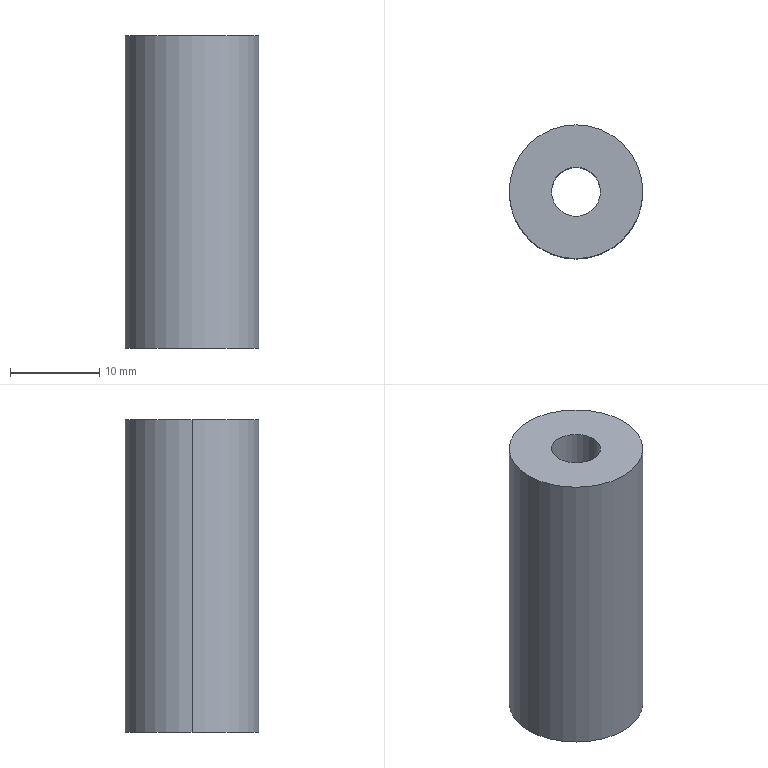Part | STEP file | track post-1 | 1 solid | 6 faces | box 15 x 15 x 35 mm | volume 5353 mm3 | cylinder 4 | plane 2 | commonest cylinder face diameters 5.5 x2 15 x2
STEP:
#1=CARTESIAN_POINT('',(0.,0.,0.));
#2=DIRECTION('',(0.,0.,1.));
#3=DIRECTION('',(1.,0.,0.));
#4=AXIS2_PLACEMENT_3D('',#1,#2,#3);
#5=CARTESIAN_POINT('',(2.75,0.,0.));
#6=VERTEX_POINT('',#5);
#7=CARTESIAN_POINT('',(2.75,0.,35.));
#8=VERTEX_POINT('',#7);
#9=CARTESIAN_POINT('',(2.75,0.,35.));
#10=DIRECTION('',(0.,0.,1.));
#11=VECTOR('',#10,1.);
#12=LINE('',#9,#11);
#13=CARTESIAN_POINT('',(0.,0.,35.));
#14=DIRECTION('',(0.,0.,1.));
#15=DIRECTION('',(1.,0.,0.));
#16=AXIS2_PLACEMENT_3D('',#13,#14,#15);
#17=CYLINDRICAL_SURFACE('',#16,2.75);
#18=CARTESIAN_POINT('',(6.283,0.));
#19=DIRECTION('',(0.,1.));
#20=VECTOR('',#19,1.);
#21=LINE('',#18,#20);
#22=(GEOMETRIC_REPRESENTATION_CONTEXT(2)PARAMETRIC_REPRESENTATION_CONTEXT()REPRESENTATION_CONTEXT('',''));
#23=DEFINITIONAL_REPRESENTATION('',(#21),#22);
#24=PCURVE('',#17,#23);
#25=CARTESIAN_POINT('',(0.,0.,35.));
#26=DIRECTION('',(0.,0.,1.));
#27=DIRECTION('',(1.,0.,0.));
#28=AXIS2_PLACEMENT_3D('',#25,#26,#27);
#29=CYLINDRICAL_SURFACE('',#28,2.75);
#30=CARTESIAN_POINT('',(0.,0.));
#31=DIRECTION('',(0.,1.));
#32=VECTOR('',#31,1.);
#33=LINE('',#30,#32);
#34=(GEOMETRIC_REPRESENTATION_CONTEXT(2)PARAMETRIC_REPRESENTATION_CONTEXT()REPRESENTATION_CONTEXT('',''));
#35=DEFINITIONAL_REPRESENTATION('',(#33),#34);
#36=PCURVE('',#29,#35);
#37=SURFACE_CURVE('',#12,(#24,#36),.PCURVE_S1.);
#38=EDGE_CURVE('',#6,#8,#37,.T.);
#39=ORIENTED_EDGE('',*,*,#38,.T.);
#40=CARTESIAN_POINT('',(-2.75,0.,35.));
#41=VERTEX_POINT('',#40);
#42=CARTESIAN_POINT('',(0.,0.,35.));
#43=DIRECTION('',(0.,0.,1.));
#44=DIRECTION('',(1.,0.,0.));
#45=AXIS2_PLACEMENT_3D('',#42,#43,#44);
#46=CIRCLE('',#45,2.75);
#47=CARTESIAN_POINT('',(0.,0.));
#48=DIRECTION('',(1.,0.));
#49=VECTOR('',#48,1.);
#50=LINE('',#47,#49);
#51=(GEOMETRIC_REPRESENTATION_CONTEXT(2)PARAMETRIC_REPRESENTATION_CONTEXT()REPRESENTATION_CONTEXT('',''));
#52=DEFINITIONAL_REPRESENTATION('',(#50),#51);
#53=PCURVE('',#17,#52);
#54=CARTESIAN_POINT('',(0.,0.,35.));
#55=DIRECTION('',(0.,0.,1.));
#56=DIRECTION('',(1.,0.,0.));
#57=AXIS2_PLACEMENT_3D('',#54,#55,#56);
#58=PLANE('',#57);
#59=CARTESIAN_POINT('',(0.,0.));
#60=DIRECTION('',(1.,0.));
#61=AXIS2_PLACEMENT_2D('',#59,#60);
#62=CIRCLE('',#61,2.75);
#63=(GEOMETRIC_REPRESENTATION_CONTEXT(2)PARAMETRIC_REPRESENTATION_CONTEXT()REPRESENTATION_CONTEXT('',''));
#64=DEFINITIONAL_REPRESENTATION('',(#62),#63);
#65=PCURVE('',#58,#64);
#66=SURFACE_CURVE('',#46,(#53,#65),.PCURVE_S1.);
#67=EDGE_CURVE('',#41,#8,#66,.T.);
#68=ORIENTED_EDGE('',*,*,#67,.F.);
#69=CARTESIAN_POINT('',(-2.75,0.,0.));
#70=VERTEX_POINT('',#69);
#71=CARTESIAN_POINT('',(-2.75,0.,35.));
#72=DIRECTION('',(0.,0.,1.));
#73=VECTOR('',#72,1.);
#74=LINE('',#71,#73);
#75=CARTESIAN_POINT('',(3.142,0.));
#76=DIRECTION('',(0.,1.));
#77=VECTOR('',#76,1.);
#78=LINE('',#75,#77);
#79=(GEOMETRIC_REPRESENTATION_CONTEXT(2)PARAMETRIC_REPRESENTATION_CONTEXT()REPRESENTATION_CONTEXT('',''));
#80=DEFINITIONAL_REPRESENTATION('',(#78),#79);
#81=PCURVE('',#17,#80);
#82=CARTESIAN_POINT('',(3.142,0.));
#83=DIRECTION('',(0.,1.));
#84=VECTOR('',#83,1.);
#85=LINE('',#82,#84);
#86=(GEOMETRIC_REPRESENTATION_CONTEXT(2)PARAMETRIC_REPRESENTATION_CONTEXT()REPRESENTATION_CONTEXT('',''));
#87=DEFINITIONAL_REPRESENTATION('',(#85),#86);
#88=PCURVE('',#29,#87);
#89=SURFACE_CURVE('',#74,(#81,#88),.PCURVE_S1.);
#90=EDGE_CURVE('',#70,#41,#89,.T.);
#91=ORIENTED_EDGE('',*,*,#90,.F.);
#92=CARTESIAN_POINT('',(0.,0.,0.));
#93=DIRECTION('',(0.,0.,1.));
#94=DIRECTION('',(1.,0.,0.));
#95=AXIS2_PLACEMENT_3D('',#92,#93,#94);
#96=CIRCLE('',#95,2.75);
#97=CARTESIAN_POINT('',(0.,-35.));
#98=DIRECTION('',(1.,0.));
#99=VECTOR('',#98,1.);
#100=LINE('',#97,#99);
#101=(GEOMETRIC_REPRESENTATION_CONTEXT(2)PARAMETRIC_REPRESENTATION_CONTEXT()REPRESENTATION_CONTEXT('',''));
#102=DEFINITIONAL_REPRESENTATION('',(#100),#101);
#103=PCURVE('',#17,#102);
#104=CARTESIAN_POINT('',(0.,0.,0.));
#105=DIRECTION('',(0.,0.,1.));
#106=DIRECTION('',(1.,0.,0.));
#107=AXIS2_PLACEMENT_3D('',#104,#105,#106);
#108=PLANE('',#107);
#109=CARTESIAN_POINT('',(0.,0.));
#110=DIRECTION('',(1.,0.));
#111=AXIS2_PLACEMENT_2D('',#109,#110);
#112=CIRCLE('',#111,2.75);
#113=(GEOMETRIC_REPRESENTATION_CONTEXT(2)PARAMETRIC_REPRESENTATION_CONTEXT()REPRESENTATION_CONTEXT('',''));
#114=DEFINITIONAL_REPRESENTATION('',(#112),#113);
#115=PCURVE('',#108,#114);
#116=SURFACE_CURVE('',#96,(#103,#115),.PCURVE_S1.);
#117=EDGE_CURVE('',#70,#6,#116,.T.);
#118=ORIENTED_EDGE('',*,*,#117,.T.);
#119=EDGE_LOOP('',(#39,#68,#91,#118));
#120=FACE_BOUND('',#119,.F.);
#121=ADVANCED_FACE('',(#120),#17,.F.);
#122=CARTESIAN_POINT('',(7.5,0.,35.));
#123=VERTEX_POINT('',#122);
#124=CARTESIAN_POINT('',(-7.5,0.,35.));
#125=VERTEX_POINT('',#124);
#126=CARTESIAN_POINT('',(0.,0.,35.));
#127=DIRECTION('',(0.,0.,1.));
#128=DIRECTION('',(1.,0.,0.));
#129=AXIS2_PLACEMENT_3D('',#126,#127,#128);
#130=CIRCLE('',#129,7.5);
#131=CARTESIAN_POINT('',(0.,0.,35.));
#132=DIRECTION('',(0.,0.,-1.));
#133=DIRECTION('',(-1.,0.,0.));
#134=AXIS2_PLACEMENT_3D('',#131,#132,#133);
#135=CYLINDRICAL_SURFACE('',#134,7.5);
#136=CARTESIAN_POINT('',(3.142,0.));
#137=DIRECTION('',(-1.,0.));
#138=VECTOR('',#137,1.);
#139=LINE('',#136,#138);
#140=(GEOMETRIC_REPRESENTATION_CONTEXT(2)PARAMETRIC_REPRESENTATION_CONTEXT()REPRESENTATION_CONTEXT('',''));
#141=DEFINITIONAL_REPRESENTATION('',(#139),#140);
#142=PCURVE('',#135,#141);
#143=CARTESIAN_POINT('',(0.,0.));
#144=DIRECTION('',(1.,0.));
#145=AXIS2_PLACEMENT_2D('',#143,#144);
#146=CIRCLE('',#145,7.5);
#147=(GEOMETRIC_REPRESENTATION_CONTEXT(2)PARAMETRIC_REPRESENTATION_CONTEXT()REPRESENTATION_CONTEXT('',''));
#148=DEFINITIONAL_REPRESENTATION('',(#146),#147);
#149=PCURVE('',#58,#148);
#150=SURFACE_CURVE('',#130,(#142,#149),.PCURVE_S1.);
#151=EDGE_CURVE('',#123,#125,#150,.T.);
#152=ORIENTED_EDGE('',*,*,#151,.F.);
#153=CARTESIAN_POINT('',(7.5,0.,0.));
#154=VERTEX_POINT('',#153);
#155=CARTESIAN_POINT('',(7.5,0.,35.));
#156=DIRECTION('',(0.,0.,-1.));
#157=VECTOR('',#156,1.);
#158=LINE('',#155,#157);
#159=CARTESIAN_POINT('',(3.142,0.));
#160=DIRECTION('',(0.,1.));
#161=VECTOR('',#160,1.);
#162=LINE('',#159,#161);
#163=(GEOMETRIC_REPRESENTATION_CONTEXT(2)PARAMETRIC_REPRESENTATION_CONTEXT()REPRESENTATION_CONTEXT('',''));
#164=DEFINITIONAL_REPRESENTATION('',(#162),#163);
#165=PCURVE('',#135,#164);
#166=CARTESIAN_POINT('',(0.,0.,35.));
#167=DIRECTION('',(0.,0.,-1.));
#168=DIRECTION('',(-1.,0.,0.));
#169=AXIS2_PLACEMENT_3D('',#166,#167,#168);
#170=CYLINDRICAL_SURFACE('',#169,7.5);
#171=CARTESIAN_POINT('',(3.142,0.));
#172=DIRECTION('',(0.,1.));
#173=VECTOR('',#172,1.);
#174=LINE('',#171,#173);
#175=(GEOMETRIC_REPRESENTATION_CONTEXT(2)PARAMETRIC_REPRESENTATION_CONTEXT()REPRESENTATION_CONTEXT('',''));
#176=DEFINITIONAL_REPRESENTATION('',(#174),#175);
#177=PCURVE('',#170,#176);
#178=SURFACE_CURVE('',#158,(#165,#177),.PCURVE_S1.);
#179=EDGE_CURVE('',#123,#154,#178,.T.);
#180=ORIENTED_EDGE('',*,*,#179,.T.);
#181=CARTESIAN_POINT('',(-7.5,0.,0.));
#182=VERTEX_POINT('',#181);
#183=CARTESIAN_POINT('',(0.,0.,0.));
#184=DIRECTION('',(0.,0.,1.));
#185=DIRECTION('',(1.,0.,0.));
#186=AXIS2_PLACEMENT_3D('',#183,#184,#185);
#187=CIRCLE('',#186,7.5);
#188=CARTESIAN_POINT('',(3.142,35.));
#189=DIRECTION('',(-1.,0.));
#190=VECTOR('',#189,1.);
#191=LINE('',#188,#190);
#192=(GEOMETRIC_REPRESENTATION_CONTEXT(2)PARAMETRIC_REPRESENTATION_CONTEXT()REPRESENTATION_CONTEXT('',''));
#193=DEFINITIONAL_REPRESENTATION('',(#191),#192);
#194=PCURVE('',#135,#193);
#195=CARTESIAN_POINT('',(0.,0.));
#196=DIRECTION('',(1.,0.));
#197=AXIS2_PLACEMENT_2D('',#195,#196);
#198=CIRCLE('',#197,7.5);
#199=(GEOMETRIC_REPRESENTATION_CONTEXT(2)PARAMETRIC_REPRESENTATION_CONTEXT()REPRESENTATION_CONTEXT('',''));
#200=DEFINITIONAL_REPRESENTATION('',(#198),#199);
#201=PCURVE('',#108,#200);
#202=SURFACE_CURVE('',#187,(#194,#201),.PCURVE_S1.);
#203=EDGE_CURVE('',#154,#182,#202,.T.);
#204=ORIENTED_EDGE('',*,*,#203,.T.);
#205=CARTESIAN_POINT('',(-7.5,0.,35.));
#206=DIRECTION('',(0.,0.,-1.));
#207=VECTOR('',#206,1.);
#208=LINE('',#205,#207);
#209=CARTESIAN_POINT('',(0.,0.));
#210=DIRECTION('',(0.,1.));
#211=VECTOR('',#210,1.);
#212=LINE('',#209,#211);
#213=(GEOMETRIC_REPRESENTATION_CONTEXT(2)PARAMETRIC_REPRESENTATION_CONTEXT()REPRESENTATION_CONTEXT('',''));
#214=DEFINITIONAL_REPRESENTATION('',(#212),#213);
#215=PCURVE('',#135,#214);
#216=CARTESIAN_POINT('',(6.283,0.));
#217=DIRECTION('',(0.,1.));
#218=VECTOR('',#217,1.);
#219=LINE('',#216,#218);
#220=(GEOMETRIC_REPRESENTATION_CONTEXT(2)PARAMETRIC_REPRESENTATION_CONTEXT()REPRESENTATION_CONTEXT('',''));
#221=DEFINITIONAL_REPRESENTATION('',(#219),#220);
#222=PCURVE('',#170,#221);
#223=SURFACE_CURVE('',#208,(#215,#222),.PCURVE_S1.);
#224=EDGE_CURVE('',#125,#182,#223,.T.);
#225=ORIENTED_EDGE('',*,*,#224,.F.);
#226=EDGE_LOOP('',(#152,#180,#204,#225));
#227=FACE_BOUND('',#226,.T.);
#228=ADVANCED_FACE('',(#227),#135,.T.);
#229=ORIENTED_EDGE('',*,*,#179,.F.);
#230=CARTESIAN_POINT('',(0.,0.,35.));
#231=DIRECTION('',(0.,0.,1.));
#232=DIRECTION('',(1.,0.,0.));
#233=AXIS2_PLACEMENT_3D('',#230,#231,#232);
#234=CIRCLE('',#233,7.5);
#235=CARTESIAN_POINT('',(9.425,0.));
#236=DIRECTION('',(-1.,0.));
#237=VECTOR('',#236,1.);
#238=LINE('',#235,#237);
#239=(GEOMETRIC_REPRESENTATION_CONTEXT(2)PARAMETRIC_REPRESENTATION_CONTEXT()REPRESENTATION_CONTEXT('',''));
#240=DEFINITIONAL_REPRESENTATION('',(#238),#239);
#241=PCURVE('',#170,#240);
#242=CARTESIAN_POINT('',(0.,0.));
#243=DIRECTION('',(1.,0.));
#244=AXIS2_PLACEMENT_2D('',#242,#243);
#245=CIRCLE('',#244,7.5);
#246=(GEOMETRIC_REPRESENTATION_CONTEXT(2)PARAMETRIC_REPRESENTATION_CONTEXT()REPRESENTATION_CONTEXT('',''));
#247=DEFINITIONAL_REPRESENTATION('',(#245),#246);
#248=PCURVE('',#58,#247);
#249=SURFACE_CURVE('',#234,(#241,#248),.PCURVE_S1.);
#250=EDGE_CURVE('',#125,#123,#249,.T.);
#251=ORIENTED_EDGE('',*,*,#250,.F.);
#252=ORIENTED_EDGE('',*,*,#224,.T.);
#253=CARTESIAN_POINT('',(0.,0.,0.));
#254=DIRECTION('',(0.,0.,1.));
#255=DIRECTION('',(1.,0.,0.));
#256=AXIS2_PLACEMENT_3D('',#253,#254,#255);
#257=CIRCLE('',#256,7.5);
#258=CARTESIAN_POINT('',(9.425,35.));
#259=DIRECTION('',(-1.,0.));
#260=VECTOR('',#259,1.);
#261=LINE('',#258,#260);
#262=(GEOMETRIC_REPRESENTATION_CONTEXT(2)PARAMETRIC_REPRESENTATION_CONTEXT()REPRESENTATION_CONTEXT('',''));
#263=DEFINITIONAL_REPRESENTATION('',(#261),#262);
#264=PCURVE('',#170,#263);
#265=CARTESIAN_POINT('',(0.,0.));
#266=DIRECTION('',(1.,0.));
#267=AXIS2_PLACEMENT_2D('',#265,#266);
#268=CIRCLE('',#267,7.5);
#269=(GEOMETRIC_REPRESENTATION_CONTEXT(2)PARAMETRIC_REPRESENTATION_CONTEXT()REPRESENTATION_CONTEXT('',''));
#270=DEFINITIONAL_REPRESENTATION('',(#268),#269);
#271=PCURVE('',#108,#270);
#272=SURFACE_CURVE('',#257,(#264,#271),.PCURVE_S1.);
#273=EDGE_CURVE('',#182,#154,#272,.T.);
#274=ORIENTED_EDGE('',*,*,#273,.T.);
#275=EDGE_LOOP('',(#229,#251,#252,#274));
#276=FACE_BOUND('',#275,.T.);
#277=ADVANCED_FACE('',(#276),#170,.T.);
#278=CARTESIAN_POINT('',(0.,0.,35.));
#279=DIRECTION('',(0.,0.,1.));
#280=DIRECTION('',(1.,0.,0.));
#281=AXIS2_PLACEMENT_3D('',#278,#279,#280);
#282=CIRCLE('',#281,2.75);
#283=CARTESIAN_POINT('',(0.,0.));
#284=DIRECTION('',(1.,0.));
#285=AXIS2_PLACEMENT_2D('',#283,#284);
#286=CIRCLE('',#285,2.75);
#287=(GEOMETRIC_REPRESENTATION_CONTEXT(2)PARAMETRIC_REPRESENTATION_CONTEXT()REPRESENTATION_CONTEXT('',''));
#288=DEFINITIONAL_REPRESENTATION('',(#286),#287);
#289=PCURVE('',#58,#288);
#290=CARTESIAN_POINT('',(0.,0.));
#291=DIRECTION('',(1.,0.));
#292=VECTOR('',#291,1.);
#293=LINE('',#290,#292);
#294=(GEOMETRIC_REPRESENTATION_CONTEXT(2)PARAMETRIC_REPRESENTATION_CONTEXT()REPRESENTATION_CONTEXT('',''));
#295=DEFINITIONAL_REPRESENTATION('',(#293),#294);
#296=PCURVE('',#29,#295);
#297=SURFACE_CURVE('',#282,(#289,#296),.PCURVE_S1.);
#298=EDGE_CURVE('',#8,#41,#297,.T.);
#299=ORIENTED_EDGE('',*,*,#298,.F.);
#300=ORIENTED_EDGE('',*,*,#67,.F.);
#301=EDGE_LOOP('',(#299,#300));
#302=FACE_BOUND('',#301,.T.);
#303=ORIENTED_EDGE('',*,*,#250,.T.);
#304=ORIENTED_EDGE('',*,*,#151,.T.);
#305=EDGE_LOOP('',(#303,#304));
#306=FACE_BOUND('',#305,.T.);
#307=ADVANCED_FACE('',(#302,#306),#58,.T.);
#308=CARTESIAN_POINT('',(0.,0.,0.));
#309=DIRECTION('',(0.,0.,1.));
#310=DIRECTION('',(1.,0.,0.));
#311=AXIS2_PLACEMENT_3D('',#308,#309,#310);
#312=CIRCLE('',#311,2.75);
#313=CARTESIAN_POINT('',(0.,0.));
#314=DIRECTION('',(1.,0.));
#315=AXIS2_PLACEMENT_2D('',#313,#314);
#316=CIRCLE('',#315,2.75);
#317=(GEOMETRIC_REPRESENTATION_CONTEXT(2)PARAMETRIC_REPRESENTATION_CONTEXT()REPRESENTATION_CONTEXT('',''));
#318=DEFINITIONAL_REPRESENTATION('',(#316),#317);
#319=PCURVE('',#108,#318);
#320=CARTESIAN_POINT('',(0.,-35.));
#321=DIRECTION('',(1.,0.));
#322=VECTOR('',#321,1.);
#323=LINE('',#320,#322);
#324=(GEOMETRIC_REPRESENTATION_CONTEXT(2)PARAMETRIC_REPRESENTATION_CONTEXT()REPRESENTATION_CONTEXT('',''));
#325=DEFINITIONAL_REPRESENTATION('',(#323),#324);
#326=PCURVE('',#29,#325);
#327=SURFACE_CURVE('',#312,(#319,#326),.PCURVE_S1.);
#328=EDGE_CURVE('',#6,#70,#327,.T.);
#329=ORIENTED_EDGE('',*,*,#328,.T.);
#330=ORIENTED_EDGE('',*,*,#117,.T.);
#331=EDGE_LOOP('',(#329,#330));
#332=FACE_BOUND('',#331,.T.);
#333=ORIENTED_EDGE('',*,*,#273,.F.);
#334=ORIENTED_EDGE('',*,*,#203,.F.);
#335=EDGE_LOOP('',(#333,#334));
#336=FACE_BOUND('',#335,.T.);
#337=ADVANCED_FACE('',(#332,#336),#108,.F.);
#338=ORIENTED_EDGE('',*,*,#298,.F.);
#339=ORIENTED_EDGE('',*,*,#38,.F.);
#340=ORIENTED_EDGE('',*,*,#328,.T.);
#341=ORIENTED_EDGE('',*,*,#90,.T.);
#342=EDGE_LOOP('',(#338,#339,#340,#341));
#343=FACE_BOUND('',#342,.F.);
#344=ADVANCED_FACE('',(#343),#29,.F.);
#345=CLOSED_SHELL('',(#121,#228,#277,#307,#337,#344));
#346=MANIFOLD_SOLID_BREP('',#345);
#347=(LENGTH_UNIT()NAMED_UNIT(*)SI_UNIT(.MILLI.,.METRE.));
#348=UNCERTAINTY_MEASURE_WITH_UNIT(LENGTH_MEASURE(0.0000001),#347,'','');
#349=(NAMED_UNIT(*)PLANE_ANGLE_UNIT()SI_UNIT($,.RADIAN.));
#350=(NAMED_UNIT(*)SI_UNIT($,.STERADIAN.)SOLID_ANGLE_UNIT());
#351=(GEOMETRIC_REPRESENTATION_CONTEXT(3)GLOBAL_UNCERTAINTY_ASSIGNED_CONTEXT((#348))GLOBAL_UNIT_ASSIGNED_CONTEXT((#347,#349,#350))REPRESENTATION_CONTEXT('',''));
#352=ADVANCED_BREP_SHAPE_REPRESENTATION('',(#4,#346),#351);